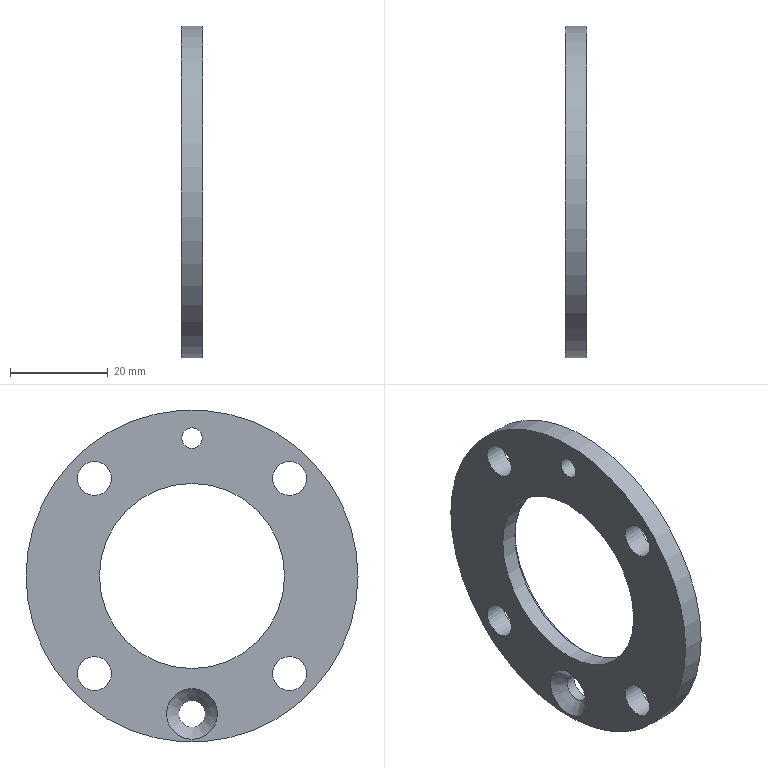Part | NX | features 2 2 | 1 solid | 12 faces | box 4.5 x 68 x 68 mm | volume 10241 mm3 | cylinder 8 | plane 2 | torus 1 | cone 1 | commonest cylinder face diameters 7 x4 4.2 x1 5.5 x1 37.9 x1 68 x1
STEP:
#1=CARTESIAN_POINT('',(-1489.5,-474.,-300.));
#2=VERTEX_POINT('',#1);
#3=CARTESIAN_POINT('',(-1489.5,-440.,-300.));
#4=DIRECTION('',(1.,0.,0.));
#5=DIRECTION('',(0.,-1.,0.));
#6=AXIS2_PLACEMENT_3D('',#3,#4,#5);
#7=CIRCLE('',#6,34.);
#8=EDGE_CURVE('',#2,#2,#7,.T.);
#9=ORIENTED_EDGE('',*,*,#8,.F.);
#10=EDGE_LOOP('',(#9));
#11=FACE_BOUND('',#10,.T.);
#12=CARTESIAN_POINT('',(-1494.,-474.,-300.));
#13=VERTEX_POINT('',#12);
#14=CARTESIAN_POINT('',(-1494.,-440.,-300.));
#15=DIRECTION('',(-1.,0.,0.));
#16=DIRECTION('',(0.,-1.,0.));
#17=AXIS2_PLACEMENT_3D('',#14,#15,#16);
#18=CIRCLE('',#17,34.);
#19=EDGE_CURVE('',#13,#13,#18,.T.);
#20=ORIENTED_EDGE('',*,*,#19,.F.);
#21=EDGE_LOOP('',(#20));
#22=FACE_BOUND('',#21,.T.);
#23=CARTESIAN_POINT('',(-1489.5,-440.,-300.));
#24=DIRECTION('',(1.,0.,0.));
#25=DIRECTION('',(0.,1.,0.));
#26=AXIS2_PLACEMENT_3D('',#23,#24,#25);
#27=CYLINDRICAL_SURFACE('',#26,34.);
#28=ADVANCED_FACE('',(#11,#22),#27,.T.);
#29=CARTESIAN_POINT('',(-1490.5,-458.95,-300.));
#30=VERTEX_POINT('',#29);
#31=CARTESIAN_POINT('',(-1490.5,-440.,-300.));
#32=DIRECTION('',(-1.,0.,0.));
#33=DIRECTION('',(0.,-1.,0.));
#34=AXIS2_PLACEMENT_3D('',#31,#32,#33);
#35=CIRCLE('',#34,18.95);
#36=EDGE_CURVE('',#30,#30,#35,.T.);
#37=ORIENTED_EDGE('',*,*,#36,.F.);
#38=EDGE_LOOP('',(#37));
#39=FACE_BOUND('',#38,.T.);
#40=CARTESIAN_POINT('',(-1494.,-458.95,-300.));
#41=VERTEX_POINT('',#40);
#42=CARTESIAN_POINT('',(-1494.,-440.,-300.));
#43=DIRECTION('',(-1.,0.,0.));
#44=DIRECTION('',(0.,-1.,0.));
#45=AXIS2_PLACEMENT_3D('',#42,#43,#44);
#46=CIRCLE('',#45,18.95);
#47=EDGE_CURVE('',#41,#41,#46,.T.);
#48=ORIENTED_EDGE('',*,*,#47,.T.);
#49=EDGE_LOOP('',(#48));
#50=FACE_BOUND('',#49,.T.);
#51=CARTESIAN_POINT('',(-1503.,-440.,-300.));
#52=DIRECTION('',(-1.,0.,0.));
#53=DIRECTION('',(0.,-1.,0.));
#54=AXIS2_PLACEMENT_3D('',#51,#52,#53);
#55=CYLINDRICAL_SURFACE('',#54,18.95);
#56=ADVANCED_FACE('',(#39,#50),#55,.F.);
#57=CARTESIAN_POINT('',(-1489.5,-423.5,-320.));
#58=VERTEX_POINT('',#57);
#59=CARTESIAN_POINT('',(-1489.5,-420.,-320.));
#60=DIRECTION('',(1.,0.,0.));
#61=DIRECTION('',(0.,-1.,0.));
#62=AXIS2_PLACEMENT_3D('',#59,#60,#61);
#63=CIRCLE('',#62,3.5);
#64=EDGE_CURVE('',#58,#58,#63,.T.);
#65=ORIENTED_EDGE('',*,*,#64,.T.);
#66=EDGE_LOOP('',(#65));
#67=FACE_BOUND('',#66,.T.);
#68=CARTESIAN_POINT('',(-1494.,-423.5,-320.));
#69=VERTEX_POINT('',#68);
#70=CARTESIAN_POINT('',(-1494.,-420.,-320.));
#71=DIRECTION('',(-1.,0.,0.));
#72=DIRECTION('',(0.,-1.,0.));
#73=AXIS2_PLACEMENT_3D('',#70,#71,#72);
#74=CIRCLE('',#73,3.5);
#75=EDGE_CURVE('',#69,#69,#74,.T.);
#76=ORIENTED_EDGE('',*,*,#75,.T.);
#77=EDGE_LOOP('',(#76));
#78=FACE_BOUND('',#77,.T.);
#79=CARTESIAN_POINT('',(-1503.,-420.,-320.));
#80=DIRECTION('',(-1.,0.,0.));
#81=DIRECTION('',(0.,-1.,0.));
#82=AXIS2_PLACEMENT_3D('',#79,#80,#81);
#83=CYLINDRICAL_SURFACE('',#82,3.5);
#84=ADVANCED_FACE('',(#67,#78),#83,.F.);
#85=CARTESIAN_POINT('',(-1489.5,-423.5,-280.));
#86=VERTEX_POINT('',#85);
#87=CARTESIAN_POINT('',(-1489.5,-420.,-280.));
#88=DIRECTION('',(1.,0.,0.));
#89=DIRECTION('',(0.,-1.,0.));
#90=AXIS2_PLACEMENT_3D('',#87,#88,#89);
#91=CIRCLE('',#90,3.5);
#92=EDGE_CURVE('',#86,#86,#91,.T.);
#93=ORIENTED_EDGE('',*,*,#92,.T.);
#94=EDGE_LOOP('',(#93));
#95=FACE_BOUND('',#94,.T.);
#96=CARTESIAN_POINT('',(-1494.,-423.5,-280.));
#97=VERTEX_POINT('',#96);
#98=CARTESIAN_POINT('',(-1494.,-420.,-280.));
#99=DIRECTION('',(-1.,0.,0.));
#100=DIRECTION('',(0.,-1.,0.));
#101=AXIS2_PLACEMENT_3D('',#98,#99,#100);
#102=CIRCLE('',#101,3.5);
#103=EDGE_CURVE('',#97,#97,#102,.T.);
#104=ORIENTED_EDGE('',*,*,#103,.T.);
#105=EDGE_LOOP('',(#104));
#106=FACE_BOUND('',#105,.T.);
#107=CARTESIAN_POINT('',(-1503.,-420.,-280.));
#108=DIRECTION('',(-1.,0.,0.));
#109=DIRECTION('',(0.,-1.,0.));
#110=AXIS2_PLACEMENT_3D('',#107,#108,#109);
#111=CYLINDRICAL_SURFACE('',#110,3.5);
#112=ADVANCED_FACE('',(#95,#106),#111,.F.);
#113=CARTESIAN_POINT('',(-1489.5,-463.5,-320.));
#114=VERTEX_POINT('',#113);
#115=CARTESIAN_POINT('',(-1489.5,-460.,-320.));
#116=DIRECTION('',(1.,0.,0.));
#117=DIRECTION('',(0.,-1.,0.));
#118=AXIS2_PLACEMENT_3D('',#115,#116,#117);
#119=CIRCLE('',#118,3.5);
#120=EDGE_CURVE('',#114,#114,#119,.T.);
#121=ORIENTED_EDGE('',*,*,#120,.T.);
#122=EDGE_LOOP('',(#121));
#123=FACE_BOUND('',#122,.T.);
#124=CARTESIAN_POINT('',(-1494.,-463.5,-320.));
#125=VERTEX_POINT('',#124);
#126=CARTESIAN_POINT('',(-1494.,-460.,-320.));
#127=DIRECTION('',(-1.,0.,0.));
#128=DIRECTION('',(0.,-1.,0.));
#129=AXIS2_PLACEMENT_3D('',#126,#127,#128);
#130=CIRCLE('',#129,3.5);
#131=EDGE_CURVE('',#125,#125,#130,.T.);
#132=ORIENTED_EDGE('',*,*,#131,.T.);
#133=EDGE_LOOP('',(#132));
#134=FACE_BOUND('',#133,.T.);
#135=CARTESIAN_POINT('',(-1503.,-460.,-320.));
#136=DIRECTION('',(-1.,0.,0.));
#137=DIRECTION('',(0.,-1.,0.));
#138=AXIS2_PLACEMENT_3D('',#135,#136,#137);
#139=CYLINDRICAL_SURFACE('',#138,3.5);
#140=ADVANCED_FACE('',(#123,#134),#139,.F.);
#141=CARTESIAN_POINT('',(-1489.5,-463.5,-280.));
#142=VERTEX_POINT('',#141);
#143=CARTESIAN_POINT('',(-1489.5,-460.,-280.));
#144=DIRECTION('',(1.,0.,0.));
#145=DIRECTION('',(0.,-1.,0.));
#146=AXIS2_PLACEMENT_3D('',#143,#144,#145);
#147=CIRCLE('',#146,3.5);
#148=EDGE_CURVE('',#142,#142,#147,.T.);
#149=ORIENTED_EDGE('',*,*,#148,.T.);
#150=EDGE_LOOP('',(#149));
#151=FACE_BOUND('',#150,.T.);
#152=CARTESIAN_POINT('',(-1494.,-463.5,-280.));
#153=VERTEX_POINT('',#152);
#154=CARTESIAN_POINT('',(-1494.,-460.,-280.));
#155=DIRECTION('',(-1.,0.,0.));
#156=DIRECTION('',(0.,-1.,0.));
#157=AXIS2_PLACEMENT_3D('',#154,#155,#156);
#158=CIRCLE('',#157,3.5);
#159=EDGE_CURVE('',#153,#153,#158,.T.);
#160=ORIENTED_EDGE('',*,*,#159,.T.);
#161=EDGE_LOOP('',(#160));
#162=FACE_BOUND('',#161,.T.);
#163=CARTESIAN_POINT('',(-1503.,-460.,-280.));
#164=DIRECTION('',(-1.,0.,0.));
#165=DIRECTION('',(0.,-1.,0.));
#166=AXIS2_PLACEMENT_3D('',#163,#164,#165);
#167=CYLINDRICAL_SURFACE('',#166,3.5);
#168=ADVANCED_FACE('',(#151,#162),#167,.F.);
#169=CARTESIAN_POINT('',(-1489.5,-420.05,-300.));
#170=VERTEX_POINT('',#169);
#171=CARTESIAN_POINT('',(-1489.5,-440.,-300.));
#172=DIRECTION('',(1.,0.,0.));
#173=DIRECTION('',(0.,1.,0.));
#174=AXIS2_PLACEMENT_3D('',#171,#172,#173);
#175=CIRCLE('',#174,19.95);
#176=EDGE_CURVE('',#170,#170,#175,.T.);
#177=ORIENTED_EDGE('',*,*,#176,.T.);
#178=EDGE_LOOP('',(#177));
#179=FACE_BOUND('',#178,.T.);
#180=ORIENTED_EDGE('',*,*,#36,.T.);
#181=EDGE_LOOP('',(#180));
#182=FACE_BOUND('',#181,.T.);
#183=CARTESIAN_POINT('',(-1489.5,-440.,-300.));
#184=DIRECTION('',(1.,0.,0.));
#185=DIRECTION('',(0.,1.,0.));
#186=AXIS2_PLACEMENT_3D('',#183,#184,#185);
#187=TOROIDAL_SURFACE('',#186,18.95,1.);
#188=ADVANCED_FACE('',(#179,#182),#187,.F.);
#189=CARTESIAN_POINT('',(-1494.,-440.,-333.45));
#190=VERTEX_POINT('',#189);
#191=CARTESIAN_POINT('',(-1494.,-440.,-328.25));
#192=DIRECTION('',(-1.,0.,0.));
#193=DIRECTION('',(0.,0.,-1.));
#194=AXIS2_PLACEMENT_3D('',#191,#192,#193);
#195=CIRCLE('',#194,5.2);
#196=EDGE_CURVE('',#190,#190,#195,.T.);
#197=ORIENTED_EDGE('',*,*,#196,.T.);
#198=EDGE_LOOP('',(#197));
#199=FACE_BOUND('',#198,.T.);
#200=CARTESIAN_POINT('',(-1491.55,-440.,-331.));
#201=VERTEX_POINT('',#200);
#202=CARTESIAN_POINT('',(-1491.55,-440.,-328.25));
#203=DIRECTION('',(1.,0.,0.));
#204=DIRECTION('',(0.,0.,-1.));
#205=AXIS2_PLACEMENT_3D('',#202,#203,#204);
#206=CIRCLE('',#205,2.75);
#207=EDGE_CURVE('',#201,#201,#206,.T.);
#208=ORIENTED_EDGE('',*,*,#207,.T.);
#209=EDGE_LOOP('',(#208));
#210=FACE_BOUND('',#209,.T.);
#211=CARTESIAN_POINT('',(-1492.775,-440.,-328.25));
#212=DIRECTION('',(-1.,0.,0.));
#213=DIRECTION('',(0.,-1.,0.));
#214=AXIS2_PLACEMENT_3D('',#211,#212,#213);
#215=CONICAL_SURFACE('',#214,3.975,0.7854);
#216=ADVANCED_FACE('',(#199,#210),#215,.F.);
#217=ORIENTED_EDGE('',*,*,#207,.F.);
#218=EDGE_LOOP('',(#217));
#219=FACE_BOUND('',#218,.T.);
#220=CARTESIAN_POINT('',(-1489.5,-440.,-331.));
#221=VERTEX_POINT('',#220);
#222=CARTESIAN_POINT('',(-1489.5,-440.,-328.25));
#223=DIRECTION('',(1.,0.,0.));
#224=DIRECTION('',(0.,0.,-1.));
#225=AXIS2_PLACEMENT_3D('',#222,#223,#224);
#226=CIRCLE('',#225,2.75);
#227=EDGE_CURVE('',#221,#221,#226,.T.);
#228=ORIENTED_EDGE('',*,*,#227,.T.);
#229=EDGE_LOOP('',(#228));
#230=FACE_BOUND('',#229,.T.);
#231=CARTESIAN_POINT('',(-1490.525,-440.,-328.25));
#232=DIRECTION('',(1.,0.,0.));
#233=DIRECTION('',(0.,1.,0.));
#234=AXIS2_PLACEMENT_3D('',#231,#232,#233);
#235=CYLINDRICAL_SURFACE('',#234,2.75);
#236=ADVANCED_FACE('',(#219,#230),#235,.F.);
#237=CARTESIAN_POINT('',(-1489.5,-440.,-269.65));
#238=VERTEX_POINT('',#237);
#239=CARTESIAN_POINT('',(-1489.5,-440.,-271.75));
#240=DIRECTION('',(1.,0.,0.));
#241=DIRECTION('',(0.,0.,1.));
#242=AXIS2_PLACEMENT_3D('',#239,#240,#241);
#243=CIRCLE('',#242,2.1);
#244=EDGE_CURVE('',#238,#238,#243,.T.);
#245=ORIENTED_EDGE('',*,*,#244,.T.);
#246=EDGE_LOOP('',(#245));
#247=FACE_BOUND('',#246,.T.);
#248=CARTESIAN_POINT('',(-1494.,-440.,-269.65));
#249=VERTEX_POINT('',#248);
#250=CARTESIAN_POINT('',(-1494.,-440.,-271.75));
#251=DIRECTION('',(-1.,0.,0.));
#252=DIRECTION('',(0.,0.,1.));
#253=AXIS2_PLACEMENT_3D('',#250,#251,#252);
#254=CIRCLE('',#253,2.1);
#255=EDGE_CURVE('',#249,#249,#254,.T.);
#256=ORIENTED_EDGE('',*,*,#255,.T.);
#257=EDGE_LOOP('',(#256));
#258=FACE_BOUND('',#257,.T.);
#259=CARTESIAN_POINT('',(-1491.75,-440.,-271.75));
#260=DIRECTION('',(-1.,0.,0.));
#261=DIRECTION('',(0.,-1.,0.));
#262=AXIS2_PLACEMENT_3D('',#259,#260,#261);
#263=CYLINDRICAL_SURFACE('',#262,2.1);
#264=ADVANCED_FACE('',(#247,#258),#263,.F.);
#265=ORIENTED_EDGE('',*,*,#255,.F.);
#266=EDGE_LOOP('',(#265));
#267=FACE_BOUND('',#266,.T.);
#268=ORIENTED_EDGE('',*,*,#196,.F.);
#269=EDGE_LOOP('',(#268));
#270=FACE_BOUND('',#269,.T.);
#271=ORIENTED_EDGE('',*,*,#159,.F.);
#272=EDGE_LOOP('',(#271));
#273=FACE_BOUND('',#272,.T.);
#274=ORIENTED_EDGE('',*,*,#131,.F.);
#275=EDGE_LOOP('',(#274));
#276=FACE_BOUND('',#275,.T.);
#277=ORIENTED_EDGE('',*,*,#103,.F.);
#278=EDGE_LOOP('',(#277));
#279=FACE_BOUND('',#278,.T.);
#280=ORIENTED_EDGE('',*,*,#75,.F.);
#281=EDGE_LOOP('',(#280));
#282=FACE_BOUND('',#281,.T.);
#283=ORIENTED_EDGE('',*,*,#47,.F.);
#284=EDGE_LOOP('',(#283));
#285=FACE_BOUND('',#284,.T.);
#286=ORIENTED_EDGE('',*,*,#19,.T.);
#287=EDGE_LOOP('',(#286));
#288=FACE_BOUND('',#287,.T.);
#289=CARTESIAN_POINT('',(-1494.,-440.,-300.));
#290=DIRECTION('',(-1.,0.,0.));
#291=DIRECTION('',(0.,-1.,0.));
#292=AXIS2_PLACEMENT_3D('',#289,#290,#291);
#293=PLANE('',#292);
#294=ADVANCED_FACE('',(#267,#270,#273,#276,#279,#282,#285,#288),#293,.T.);
#295=ORIENTED_EDGE('',*,*,#244,.F.);
#296=EDGE_LOOP('',(#295));
#297=FACE_BOUND('',#296,.T.);
#298=ORIENTED_EDGE('',*,*,#227,.F.);
#299=EDGE_LOOP('',(#298));
#300=FACE_BOUND('',#299,.T.);
#301=ORIENTED_EDGE('',*,*,#176,.F.);
#302=EDGE_LOOP('',(#301));
#303=FACE_BOUND('',#302,.T.);
#304=ORIENTED_EDGE('',*,*,#148,.F.);
#305=EDGE_LOOP('',(#304));
#306=FACE_BOUND('',#305,.T.);
#307=ORIENTED_EDGE('',*,*,#120,.F.);
#308=EDGE_LOOP('',(#307));
#309=FACE_BOUND('',#308,.T.);
#310=ORIENTED_EDGE('',*,*,#92,.F.);
#311=EDGE_LOOP('',(#310));
#312=FACE_BOUND('',#311,.T.);
#313=ORIENTED_EDGE('',*,*,#64,.F.);
#314=EDGE_LOOP('',(#313));
#315=FACE_BOUND('',#314,.T.);
#316=ORIENTED_EDGE('',*,*,#8,.T.);
#317=EDGE_LOOP('',(#316));
#318=FACE_BOUND('',#317,.T.);
#319=CARTESIAN_POINT('',(-1489.5,-440.,-300.));
#320=DIRECTION('',(-1.,0.,0.));
#321=DIRECTION('',(0.,-1.,0.));
#322=AXIS2_PLACEMENT_3D('',#319,#320,#321);
#323=PLANE('',#322);
#324=ADVANCED_FACE('',(#297,#300,#303,#306,#309,#312,#315,#318),#323,.F.);
#325=CLOSED_SHELL('',(#28,#56,#84,#112,#140,#168,#188,#216,#236,#264,#294,#324));
#326=MANIFOLD_SOLID_BREP('',#325);
#327=(LENGTH_UNIT()NAMED_UNIT(*)SI_UNIT(.MILLI.,.METRE.));
#328=UNCERTAINTY_MEASURE_WITH_UNIT(LENGTH_MEASURE(0.00001),#327,'','');
#329=(NAMED_UNIT(*)PLANE_ANGLE_UNIT()SI_UNIT($,.RADIAN.));
#330=(NAMED_UNIT(*)SI_UNIT($,.STERADIAN.)SOLID_ANGLE_UNIT());
#331=(GEOMETRIC_REPRESENTATION_CONTEXT(3)GLOBAL_UNCERTAINTY_ASSIGNED_CONTEXT((#328))GLOBAL_UNIT_ASSIGNED_CONTEXT((#327,#329,#330))REPRESENTATION_CONTEXT('',''));
#332=ADVANCED_BREP_SHAPE_REPRESENTATION('',(#326),#331);